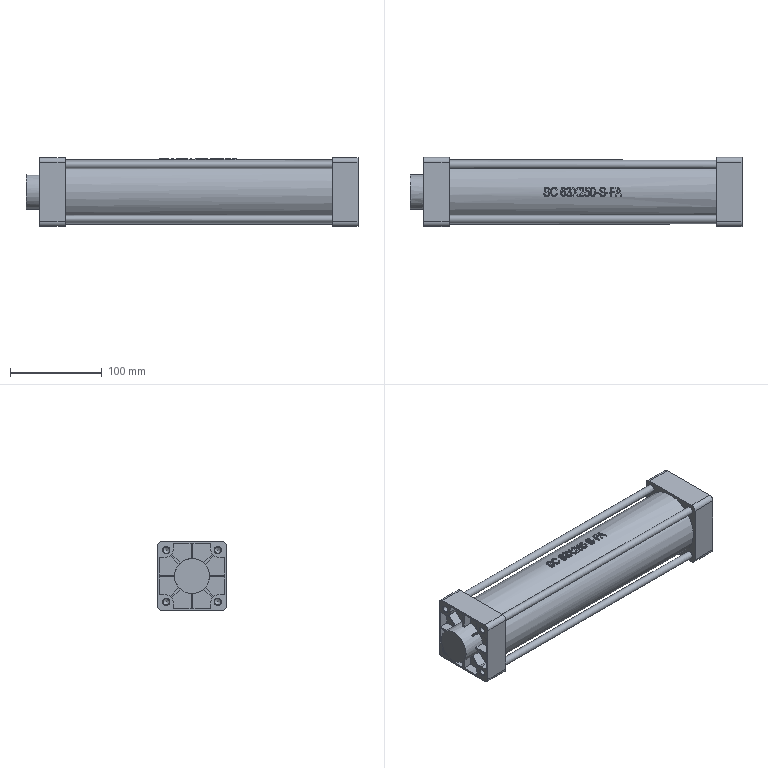Part | STEP file | Tube feed_id390_x_t | 1 solid | 252 faces | box 361 x 75 x 75 mm | volume 1441708 mm3 | plane 126 | cylinder 62 | spline 48 | cone 16 | commonest cylinder face diameters 15 x16 72 x13 38 x9 6.8 x8 10 x8 8 x4